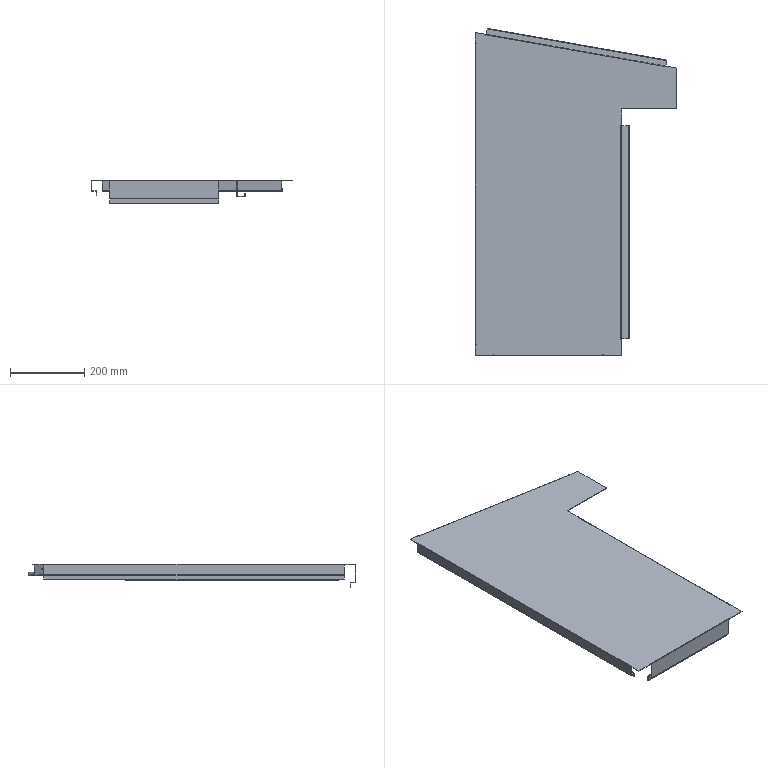Part | SolidWorks | features MirrorStock 1 | 1 solid | 148 faces | box 543 x 881.04 x 63.5 mm | volume 714708 mm3 | plane 116 | cylinder 32 | commonest cylinder face diameters 0.2 x12 3.2 x12 7 x8